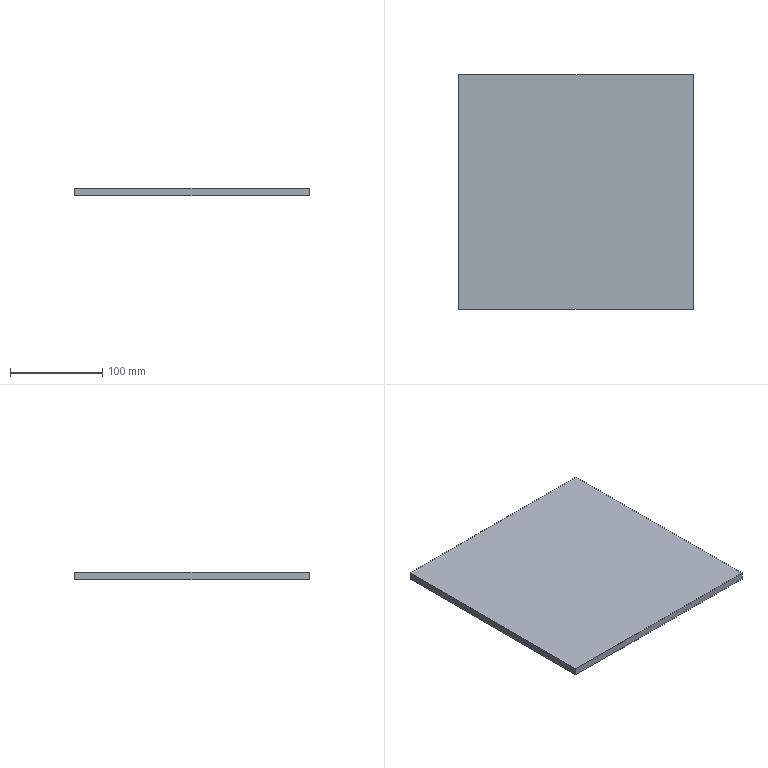Part | SolidWorks | features Extrusion 1 | 1 solid | 6 faces | box 254 x 254 x 8 mm | volume 516128 mm3 | plane 6
STEP:
#1=CARTESIAN_POINT('',(-127.,127.,-4.));
#2=VERTEX_POINT('',#1);
#3=CARTESIAN_POINT('',(-127.,-127.,-4.));
#4=VERTEX_POINT('',#3);
#5=CARTESIAN_POINT('',(-127.,127.,-4.));
#6=DIRECTION('',(0.,-1.,0.));
#7=VECTOR('',#6,1000.);
#8=LINE('',#5,#7);
#9=EDGE_CURVE('',#2,#4,#8,.T.);
#10=ORIENTED_EDGE('',*,*,#9,.T.);
#11=CARTESIAN_POINT('',(-127.,-127.,4.));
#12=VERTEX_POINT('',#11);
#13=CARTESIAN_POINT('',(-127.,-127.,4.));
#14=DIRECTION('',(0.,0.,-1.));
#15=VECTOR('',#14,1000.);
#16=LINE('',#13,#15);
#17=EDGE_CURVE('',#12,#4,#16,.T.);
#18=ORIENTED_EDGE('',*,*,#17,.F.);
#19=CARTESIAN_POINT('',(-127.,127.,4.));
#20=VERTEX_POINT('',#19);
#21=CARTESIAN_POINT('',(-127.,127.,4.));
#22=DIRECTION('',(0.,-1.,0.));
#23=VECTOR('',#22,1000.);
#24=LINE('',#21,#23);
#25=EDGE_CURVE('',#20,#12,#24,.T.);
#26=ORIENTED_EDGE('',*,*,#25,.F.);
#27=CARTESIAN_POINT('',(-127.,127.,4.));
#28=DIRECTION('',(0.,0.,-1.));
#29=VECTOR('',#28,1000.);
#30=LINE('',#27,#29);
#31=EDGE_CURVE('',#20,#2,#30,.T.);
#32=ORIENTED_EDGE('',*,*,#31,.T.);
#33=EDGE_LOOP('',(#10,#18,#26,#32));
#34=FACE_OUTER_BOUND('',#33,.T.);
#35=CARTESIAN_POINT('',(-127.,127.,4.));
#36=DIRECTION('',(1.,0.,0.));
#37=DIRECTION('',(0.,1.,0.));
#38=AXIS2_PLACEMENT_3D('',#35,#36,#37);
#39=PLANE('',#38);
#40=ADVANCED_FACE('',(#34),#39,.F.);
#41=CARTESIAN_POINT('',(127.,-127.,-4.));
#42=VERTEX_POINT('',#41);
#43=CARTESIAN_POINT('',(-127.,-127.,-4.));
#44=DIRECTION('',(1.,0.,0.));
#45=VECTOR('',#44,1000.);
#46=LINE('',#43,#45);
#47=EDGE_CURVE('',#4,#42,#46,.T.);
#48=ORIENTED_EDGE('',*,*,#47,.T.);
#49=CARTESIAN_POINT('',(127.,-127.,4.));
#50=VERTEX_POINT('',#49);
#51=CARTESIAN_POINT('',(127.,-127.,4.));
#52=DIRECTION('',(0.,0.,-1.));
#53=VECTOR('',#52,1000.);
#54=LINE('',#51,#53);
#55=EDGE_CURVE('',#50,#42,#54,.T.);
#56=ORIENTED_EDGE('',*,*,#55,.F.);
#57=CARTESIAN_POINT('',(-127.,-127.,4.));
#58=DIRECTION('',(1.,0.,0.));
#59=VECTOR('',#58,1000.);
#60=LINE('',#57,#59);
#61=EDGE_CURVE('',#12,#50,#60,.T.);
#62=ORIENTED_EDGE('',*,*,#61,.F.);
#63=ORIENTED_EDGE('',*,*,#17,.T.);
#64=EDGE_LOOP('',(#48,#56,#62,#63));
#65=FACE_OUTER_BOUND('',#64,.T.);
#66=CARTESIAN_POINT('',(-127.,-127.,4.));
#67=DIRECTION('',(0.,1.,0.));
#68=DIRECTION('',(0.,0.,1.));
#69=AXIS2_PLACEMENT_3D('',#66,#67,#68);
#70=PLANE('',#69);
#71=ADVANCED_FACE('',(#65),#70,.F.);
#72=CARTESIAN_POINT('',(127.,127.,-4.));
#73=VERTEX_POINT('',#72);
#74=CARTESIAN_POINT('',(127.,127.,-4.));
#75=DIRECTION('',(0.,1.,0.));
#76=VECTOR('',#75,1000.);
#77=LINE('',#74,#76);
#78=EDGE_CURVE('',#42,#73,#77,.T.);
#79=ORIENTED_EDGE('',*,*,#78,.T.);
#80=CARTESIAN_POINT('',(127.,127.,4.));
#81=VERTEX_POINT('',#80);
#82=CARTESIAN_POINT('',(127.,127.,4.));
#83=DIRECTION('',(0.,0.,-1.));
#84=VECTOR('',#83,1000.);
#85=LINE('',#82,#84);
#86=EDGE_CURVE('',#81,#73,#85,.T.);
#87=ORIENTED_EDGE('',*,*,#86,.F.);
#88=CARTESIAN_POINT('',(127.,127.,4.));
#89=DIRECTION('',(0.,1.,0.));
#90=VECTOR('',#89,1000.);
#91=LINE('',#88,#90);
#92=EDGE_CURVE('',#50,#81,#91,.T.);
#93=ORIENTED_EDGE('',*,*,#92,.F.);
#94=ORIENTED_EDGE('',*,*,#55,.T.);
#95=EDGE_LOOP('',(#79,#87,#93,#94));
#96=FACE_OUTER_BOUND('',#95,.T.);
#97=CARTESIAN_POINT('',(127.,127.,4.));
#98=DIRECTION('',(-1.,0.,0.));
#99=DIRECTION('',(0.,-1.,0.));
#100=AXIS2_PLACEMENT_3D('',#97,#98,#99);
#101=PLANE('',#100);
#102=ADVANCED_FACE('',(#96),#101,.F.);
#103=CARTESIAN_POINT('',(-127.,127.,-4.));
#104=DIRECTION('',(-1.,0.,0.));
#105=VECTOR('',#104,1000.);
#106=LINE('',#103,#105);
#107=EDGE_CURVE('',#73,#2,#106,.T.);
#108=ORIENTED_EDGE('',*,*,#107,.T.);
#109=ORIENTED_EDGE('',*,*,#31,.F.);
#110=CARTESIAN_POINT('',(-127.,127.,4.));
#111=DIRECTION('',(-1.,0.,0.));
#112=VECTOR('',#111,1000.);
#113=LINE('',#110,#112);
#114=EDGE_CURVE('',#81,#20,#113,.T.);
#115=ORIENTED_EDGE('',*,*,#114,.F.);
#116=ORIENTED_EDGE('',*,*,#86,.T.);
#117=EDGE_LOOP('',(#108,#109,#115,#116));
#118=FACE_OUTER_BOUND('',#117,.T.);
#119=CARTESIAN_POINT('',(-127.,127.,4.));
#120=DIRECTION('',(0.,-1.,0.));
#121=DIRECTION('',(0.,0.,-1.));
#122=AXIS2_PLACEMENT_3D('',#119,#120,#121);
#123=PLANE('',#122);
#124=ADVANCED_FACE('',(#118),#123,.F.);
#125=ORIENTED_EDGE('',*,*,#25,.T.);
#126=ORIENTED_EDGE('',*,*,#61,.T.);
#127=ORIENTED_EDGE('',*,*,#92,.T.);
#128=ORIENTED_EDGE('',*,*,#114,.T.);
#129=EDGE_LOOP('',(#125,#126,#127,#128));
#130=FACE_OUTER_BOUND('',#129,.T.);
#131=CARTESIAN_POINT('',(0.,0.,4.));
#132=DIRECTION('',(0.,0.,1.));
#133=DIRECTION('',(1.,0.,0.));
#134=AXIS2_PLACEMENT_3D('',#131,#132,#133);
#135=PLANE('',#134);
#136=ADVANCED_FACE('',(#130),#135,.T.);
#137=ORIENTED_EDGE('',*,*,#9,.F.);
#138=ORIENTED_EDGE('',*,*,#107,.F.);
#139=ORIENTED_EDGE('',*,*,#78,.F.);
#140=ORIENTED_EDGE('',*,*,#47,.F.);
#141=EDGE_LOOP('',(#137,#138,#139,#140));
#142=FACE_OUTER_BOUND('',#141,.T.);
#143=CARTESIAN_POINT('',(0.,0.,-4.));
#144=DIRECTION('',(0.,0.,1.));
#145=DIRECTION('',(1.,0.,0.));
#146=AXIS2_PLACEMENT_3D('',#143,#144,#145);
#147=PLANE('',#146);
#148=ADVANCED_FACE('',(#142),#147,.F.);
#149=CLOSED_SHELL('',(#40,#71,#102,#124,#136,#148));
#150=MANIFOLD_SOLID_BREP('',#149);
#151=CARTESIAN_POINT('',(0.,0.,0.));
#152=DIRECTION('',(0.,0.,1.));
#153=DIRECTION('',(1.,0.,0.));
#154=AXIS2_PLACEMENT_3D('',#151,#152,#153);
#155=(LENGTH_UNIT()NAMED_UNIT(*)SI_UNIT(.MILLI.,.METRE.));
#156=UNCERTAINTY_MEASURE_WITH_UNIT(LENGTH_MEASURE(0.00001),#155,'','');
#157=(NAMED_UNIT(*)PLANE_ANGLE_UNIT()SI_UNIT($,.RADIAN.));
#158=(NAMED_UNIT(*)SI_UNIT($,.STERADIAN.)SOLID_ANGLE_UNIT());
#159=(GEOMETRIC_REPRESENTATION_CONTEXT(3)GLOBAL_UNCERTAINTY_ASSIGNED_CONTEXT((#156))GLOBAL_UNIT_ASSIGNED_CONTEXT((#155,#157,#158))REPRESENTATION_CONTEXT('',''));
#160=ADVANCED_BREP_SHAPE_REPRESENTATION('',(#150,#154),#159);